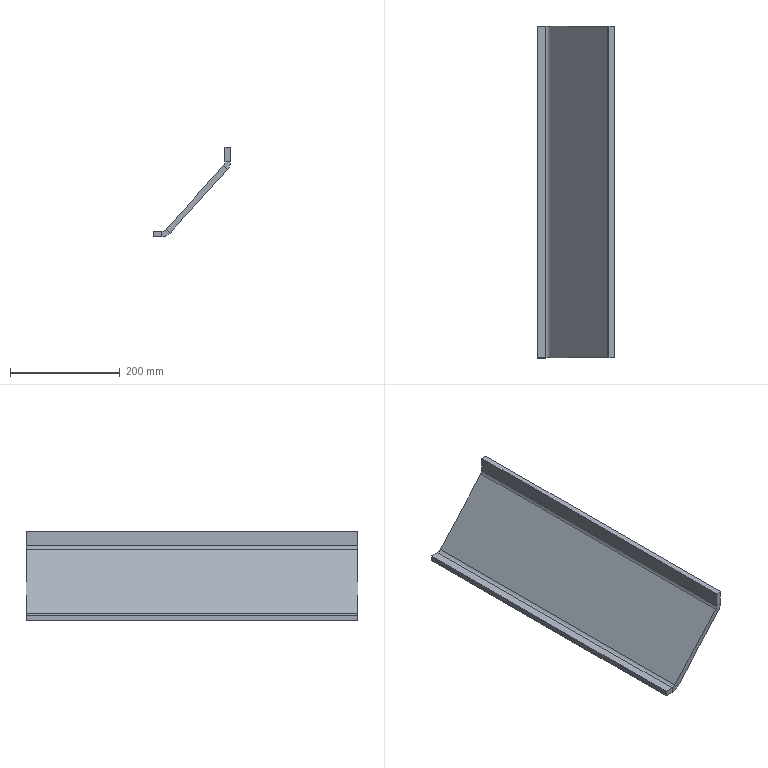Part | SolidWorks | features DelFace 1, DeleteBody 1, FlatPattern 1, FlattenBends 1, MBimport 1, ProcessBends 1, SheetMetal 1 | 1 solid | 22 faces | box 140 x 605 x 163 mm | volume 1343139 mm3 | plane 18 | cylinder 4 | commonest cylinder face diameters 20 x2 40 x2
STEP:
#1=CARTESIAN_POINT('',(500.5,-305.,-1153.));
#2=VERTEX_POINT('',#1);
#3=CARTESIAN_POINT('',(500.5,300.,-1153.));
#4=VERTEX_POINT('',#3);
#5=CARTESIAN_POINT('',(500.5,-305.,-1153.));
#6=DIRECTION('',(0.,1.,0.));
#7=VECTOR('',#6,1000.);
#8=LINE('',#5,#7);
#9=EDGE_CURVE('',#2,#4,#8,.T.);
#10=ORIENTED_EDGE('',*,*,#9,.F.);
#11=CARTESIAN_POINT('',(500.5,-305.,-1143.));
#12=VERTEX_POINT('',#11);
#13=CARTESIAN_POINT('',(500.5,-305.,67.383));
#14=DIRECTION('',(0.,0.,-1.));
#15=VECTOR('',#14,1000.);
#16=LINE('',#13,#15);
#17=EDGE_CURVE('',#12,#2,#16,.T.);
#18=ORIENTED_EDGE('',*,*,#17,.F.);
#19=CARTESIAN_POINT('',(500.5,300.,-1143.));
#20=VERTEX_POINT('',#19);
#21=CARTESIAN_POINT('',(500.5,-305.,-1143.));
#22=DIRECTION('',(0.,1.,0.));
#23=VECTOR('',#22,1000.);
#24=LINE('',#21,#23);
#25=EDGE_CURVE('',#12,#20,#24,.T.);
#26=ORIENTED_EDGE('',*,*,#25,.T.);
#27=CARTESIAN_POINT('',(500.5,300.,67.383));
#28=DIRECTION('',(0.,0.,-1.));
#29=VECTOR('',#28,1000.);
#30=LINE('',#27,#29);
#31=EDGE_CURVE('',#20,#4,#30,.T.);
#32=ORIENTED_EDGE('',*,*,#31,.T.);
#33=EDGE_LOOP('',(#10,#18,#26,#32));
#34=FACE_OUTER_BOUND('',#33,.T.);
#35=CARTESIAN_POINT('',(500.5,-305.,67.383));
#36=DIRECTION('',(-1.,0.,0.));
#37=DIRECTION('',(0.,0.,1.));
#38=AXIS2_PLACEMENT_3D('',#35,#36,#37);
#39=PLANE('',#38);
#40=ADVANCED_FACE('',(#34),#39,.T.);
#41=CARTESIAN_POINT('',(515.725,300.,-1143.));
#42=VERTEX_POINT('',#41);
#43=CARTESIAN_POINT('',(515.725,300.,-1153.));
#44=VERTEX_POINT('',#43);
#45=CARTESIAN_POINT('',(515.725,300.,67.383));
#46=DIRECTION('',(0.,0.,-1.));
#47=VECTOR('',#46,1000.);
#48=LINE('',#45,#47);
#49=EDGE_CURVE('',#42,#44,#48,.T.);
#50=ORIENTED_EDGE('',*,*,#49,.T.);
#51=CARTESIAN_POINT('',(500.5,300.,-1153.));
#52=DIRECTION('',(1.,0.,0.));
#53=VECTOR('',#52,1000.);
#54=LINE('',#51,#53);
#55=EDGE_CURVE('',#4,#44,#54,.T.);
#56=ORIENTED_EDGE('',*,*,#55,.F.);
#57=ORIENTED_EDGE('',*,*,#31,.F.);
#58=CARTESIAN_POINT('',(517.751,300.,-1143.));
#59=DIRECTION('',(-1.,0.,0.));
#60=VECTOR('',#59,1000.);
#61=LINE('',#58,#60);
#62=EDGE_CURVE('',#42,#20,#61,.T.);
#63=ORIENTED_EDGE('',*,*,#62,.F.);
#64=EDGE_LOOP('',(#50,#56,#57,#63));
#65=FACE_OUTER_BOUND('',#64,.T.);
#66=CARTESIAN_POINT('',(517.751,300.,67.383));
#67=DIRECTION('',(0.,-1.,0.));
#68=DIRECTION('',(-0.7431,0.,-0.6691));
#69=AXIS2_PLACEMENT_3D('',#66,#67,#68);
#70=PLANE('',#69);
#71=ADVANCED_FACE('',(#65),#70,.F.);
#72=ORIENTED_EDGE('',*,*,#55,.T.);
#73=CARTESIAN_POINT('',(515.725,-305.,-1153.));
#74=VERTEX_POINT('',#73);
#75=CARTESIAN_POINT('',(515.725,300.,-1153.));
#76=DIRECTION('',(0.,-1.,0.));
#77=VECTOR('',#76,1000.);
#78=LINE('',#75,#77);
#79=EDGE_CURVE('',#44,#74,#78,.T.);
#80=ORIENTED_EDGE('',*,*,#79,.T.);
#81=CARTESIAN_POINT('',(500.5,-305.,-1153.));
#82=DIRECTION('',(1.,0.,0.));
#83=VECTOR('',#82,1000.);
#84=LINE('',#81,#83);
#85=EDGE_CURVE('',#2,#74,#84,.T.);
#86=ORIENTED_EDGE('',*,*,#85,.F.);
#87=ORIENTED_EDGE('',*,*,#9,.T.);
#88=EDGE_LOOP('',(#72,#80,#86,#87));
#89=FACE_OUTER_BOUND('',#88,.T.);
#90=CARTESIAN_POINT('',(500.5,-305.,-1153.));
#91=DIRECTION('',(0.,0.,1.));
#92=DIRECTION('',(1.,0.,0.));
#93=AXIS2_PLACEMENT_3D('',#90,#91,#92);
#94=PLANE('',#93);
#95=ADVANCED_FACE('',(#89),#94,.F.);
#96=ORIENTED_EDGE('',*,*,#85,.T.);
#97=CARTESIAN_POINT('',(515.725,-305.,-1143.));
#98=VERTEX_POINT('',#97);
#99=CARTESIAN_POINT('',(515.725,-305.,67.383));
#100=DIRECTION('',(0.,0.,-1.));
#101=VECTOR('',#100,1000.);
#102=LINE('',#99,#101);
#103=EDGE_CURVE('',#98,#74,#102,.T.);
#104=ORIENTED_EDGE('',*,*,#103,.F.);
#105=CARTESIAN_POINT('',(517.751,-305.,-1143.));
#106=DIRECTION('',(1.,0.,0.));
#107=VECTOR('',#106,1000.);
#108=LINE('',#105,#107);
#109=EDGE_CURVE('',#12,#98,#108,.T.);
#110=ORIENTED_EDGE('',*,*,#109,.F.);
#111=ORIENTED_EDGE('',*,*,#17,.T.);
#112=EDGE_LOOP('',(#96,#104,#110,#111));
#113=FACE_OUTER_BOUND('',#112,.T.);
#114=CARTESIAN_POINT('',(517.751,-305.,67.383));
#115=DIRECTION('',(0.,-1.,0.));
#116=DIRECTION('',(-0.7431,0.,-0.6691));
#117=AXIS2_PLACEMENT_3D('',#114,#115,#116);
#118=PLANE('',#117);
#119=ADVANCED_FACE('',(#113),#118,.T.);
#120=ORIENTED_EDGE('',*,*,#109,.T.);
#121=CARTESIAN_POINT('',(515.725,300.,-1143.));
#122=DIRECTION('',(0.,1.,0.));
#123=VECTOR('',#122,1000.);
#124=LINE('',#121,#123);
#125=EDGE_CURVE('',#98,#42,#124,.T.);
#126=ORIENTED_EDGE('',*,*,#125,.T.);
#127=ORIENTED_EDGE('',*,*,#62,.T.);
#128=ORIENTED_EDGE('',*,*,#25,.F.);
#129=EDGE_LOOP('',(#120,#126,#127,#128));
#130=FACE_OUTER_BOUND('',#129,.T.);
#131=CARTESIAN_POINT('',(517.751,-305.,-1143.));
#132=DIRECTION('',(0.,0.,-1.));
#133=DIRECTION('',(0.,-1.,0.));
#134=AXIS2_PLACEMENT_3D('',#131,#132,#133);
#135=PLANE('',#134);
#136=ADVANCED_FACE('',(#130),#135,.F.);
#137=CARTESIAN_POINT('',(630.5,-305.,-990.));
#138=VERTEX_POINT('',#137);
#139=CARTESIAN_POINT('',(640.5,-305.,-990.));
#140=VERTEX_POINT('',#139);
#141=CARTESIAN_POINT('',(-580.672,-305.,-990.));
#142=DIRECTION('',(1.,0.,0.));
#143=VECTOR('',#142,1000.);
#144=LINE('',#141,#143);
#145=EDGE_CURVE('',#138,#140,#144,.T.);
#146=ORIENTED_EDGE('',*,*,#145,.T.);
#147=CARTESIAN_POINT('',(640.5,300.,-990.));
#148=VERTEX_POINT('',#147);
#149=CARTESIAN_POINT('',(640.5,-305.,-990.));
#150=DIRECTION('',(0.,1.,0.));
#151=VECTOR('',#150,1000.);
#152=LINE('',#149,#151);
#153=EDGE_CURVE('',#140,#148,#152,.T.);
#154=ORIENTED_EDGE('',*,*,#153,.T.);
#155=CARTESIAN_POINT('',(630.5,300.,-990.));
#156=VERTEX_POINT('',#155);
#157=CARTESIAN_POINT('',(-580.672,300.,-990.));
#158=DIRECTION('',(1.,0.,0.));
#159=VECTOR('',#158,1000.);
#160=LINE('',#157,#159);
#161=EDGE_CURVE('',#156,#148,#160,.T.);
#162=ORIENTED_EDGE('',*,*,#161,.F.);
#163=CARTESIAN_POINT('',(630.5,-305.,-990.));
#164=DIRECTION('',(0.,1.,0.));
#165=VECTOR('',#164,1000.);
#166=LINE('',#163,#165);
#167=EDGE_CURVE('',#138,#156,#166,.T.);
#168=ORIENTED_EDGE('',*,*,#167,.F.);
#169=EDGE_LOOP('',(#146,#154,#162,#168));
#170=FACE_OUTER_BOUND('',#169,.T.);
#171=CARTESIAN_POINT('',(-580.672,-305.,-990.));
#172=DIRECTION('',(0.,0.,-1.));
#173=DIRECTION('',(-1.,0.,0.));
#174=AXIS2_PLACEMENT_3D('',#171,#172,#173);
#175=PLANE('',#174);
#176=ADVANCED_FACE('',(#170),#175,.F.);
#177=CARTESIAN_POINT('',(640.5,-305.,-1016.636));
#178=VERTEX_POINT('',#177);
#179=CARTESIAN_POINT('',(640.5,-305.,-1016.314));
#180=DIRECTION('',(0.,0.,1.));
#181=VECTOR('',#180,1000.);
#182=LINE('',#179,#181);
#183=EDGE_CURVE('',#178,#140,#182,.T.);
#184=ORIENTED_EDGE('',*,*,#183,.T.);
#185=ORIENTED_EDGE('',*,*,#145,.F.);
#186=CARTESIAN_POINT('',(630.5,-305.,-1016.636));
#187=VERTEX_POINT('',#186);
#188=CARTESIAN_POINT('',(630.5,-305.,-990.));
#189=DIRECTION('',(0.,0.,-1.));
#190=VECTOR('',#189,1000.);
#191=LINE('',#188,#190);
#192=EDGE_CURVE('',#138,#187,#191,.T.);
#193=ORIENTED_EDGE('',*,*,#192,.T.);
#194=CARTESIAN_POINT('',(-580.672,-305.,-1016.636));
#195=DIRECTION('',(1.,0.,0.));
#196=VECTOR('',#195,1000.);
#197=LINE('',#194,#196);
#198=EDGE_CURVE('',#187,#178,#197,.T.);
#199=ORIENTED_EDGE('',*,*,#198,.T.);
#200=EDGE_LOOP('',(#184,#185,#193,#199));
#201=FACE_OUTER_BOUND('',#200,.T.);
#202=CARTESIAN_POINT('',(-580.672,-305.,-990.));
#203=DIRECTION('',(0.,-1.,0.));
#204=DIRECTION('',(0.6691,0.,-0.7431));
#205=AXIS2_PLACEMENT_3D('',#202,#203,#204);
#206=PLANE('',#205);
#207=ADVANCED_FACE('',(#201),#206,.T.);
#208=ORIENTED_EDGE('',*,*,#183,.F.);
#209=CARTESIAN_POINT('',(640.5,300.,-1016.636));
#210=VERTEX_POINT('',#209);
#211=CARTESIAN_POINT('',(640.5,-305.,-1016.636));
#212=DIRECTION('',(0.,1.,0.));
#213=VECTOR('',#212,1000.);
#214=LINE('',#211,#213);
#215=EDGE_CURVE('',#178,#210,#214,.T.);
#216=ORIENTED_EDGE('',*,*,#215,.T.);
#217=CARTESIAN_POINT('',(640.5,300.,-990.));
#218=DIRECTION('',(0.,0.,-1.));
#219=VECTOR('',#218,1000.);
#220=LINE('',#217,#219);
#221=EDGE_CURVE('',#148,#210,#220,.T.);
#222=ORIENTED_EDGE('',*,*,#221,.F.);
#223=ORIENTED_EDGE('',*,*,#153,.F.);
#224=EDGE_LOOP('',(#208,#216,#222,#223));
#225=FACE_OUTER_BOUND('',#224,.T.);
#226=CARTESIAN_POINT('',(640.5,-305.,-1016.314));
#227=DIRECTION('',(-1.,0.,0.));
#228=DIRECTION('',(0.,0.,1.));
#229=AXIS2_PLACEMENT_3D('',#226,#227,#228);
#230=PLANE('',#229);
#231=ADVANCED_FACE('',(#225),#230,.F.);
#232=ORIENTED_EDGE('',*,*,#161,.T.);
#233=ORIENTED_EDGE('',*,*,#221,.T.);
#234=CARTESIAN_POINT('',(630.5,300.,-1016.636));
#235=VERTEX_POINT('',#234);
#236=CARTESIAN_POINT('',(-580.672,300.,-1016.636));
#237=DIRECTION('',(1.,0.,0.));
#238=VECTOR('',#237,1000.);
#239=LINE('',#236,#238);
#240=EDGE_CURVE('',#235,#210,#239,.T.);
#241=ORIENTED_EDGE('',*,*,#240,.F.);
#242=CARTESIAN_POINT('',(630.5,300.,-990.));
#243=DIRECTION('',(0.,0.,-1.));
#244=VECTOR('',#243,1000.);
#245=LINE('',#242,#244);
#246=EDGE_CURVE('',#156,#235,#245,.T.);
#247=ORIENTED_EDGE('',*,*,#246,.F.);
#248=EDGE_LOOP('',(#232,#233,#241,#247));
#249=FACE_OUTER_BOUND('',#248,.T.);
#250=CARTESIAN_POINT('',(-580.672,300.,-990.));
#251=DIRECTION('',(0.,-1.,0.));
#252=DIRECTION('',(0.6691,0.,-0.7431));
#253=AXIS2_PLACEMENT_3D('',#250,#251,#252);
#254=PLANE('',#253);
#255=ADVANCED_FACE('',(#249),#254,.F.);
#256=ORIENTED_EDGE('',*,*,#246,.T.);
#257=CARTESIAN_POINT('',(630.5,-305.,-1016.636));
#258=DIRECTION('',(0.,-1.,0.));
#259=VECTOR('',#258,1000.);
#260=LINE('',#257,#259);
#261=EDGE_CURVE('',#235,#187,#260,.T.);
#262=ORIENTED_EDGE('',*,*,#261,.T.);
#263=ORIENTED_EDGE('',*,*,#192,.F.);
#264=ORIENTED_EDGE('',*,*,#167,.T.);
#265=EDGE_LOOP('',(#256,#262,#263,#264));
#266=FACE_OUTER_BOUND('',#265,.T.);
#267=CARTESIAN_POINT('',(630.5,-305.,-990.));
#268=DIRECTION('',(1.,0.,0.));
#269=DIRECTION('',(0.,1.,0.));
#270=AXIS2_PLACEMENT_3D('',#267,#268,#269);
#271=PLANE('',#270);
#272=ADVANCED_FACE('',(#266),#271,.F.);
#273=CARTESIAN_POINT('',(627.931,300.,-1023.327));
#274=VERTEX_POINT('',#273);
#275=CARTESIAN_POINT('',(635.363,300.,-1030.019));
#276=VERTEX_POINT('',#275);
#277=CARTESIAN_POINT('',(-300.902,300.,-187.001));
#278=DIRECTION('',(0.7431,0.,-0.6691));
#279=VECTOR('',#278,1000.);
#280=LINE('',#277,#279);
#281=EDGE_CURVE('',#274,#276,#280,.T.);
#282=ORIENTED_EDGE('',*,*,#281,.T.);
#283=CARTESIAN_POINT('',(530.588,300.,-1146.383));
#284=VERTEX_POINT('',#283);
#285=CARTESIAN_POINT('',(529.984,300.,-1147.053));
#286=DIRECTION('',(0.6691,0.,0.7431));
#287=VECTOR('',#286,1000.);
#288=LINE('',#285,#287);
#289=EDGE_CURVE('',#284,#276,#288,.T.);
#290=ORIENTED_EDGE('',*,*,#289,.F.);
#291=CARTESIAN_POINT('',(523.157,300.,-1139.691));
#292=VERTEX_POINT('',#291);
#293=CARTESIAN_POINT('',(-405.677,300.,-303.365));
#294=DIRECTION('',(0.7431,0.,-0.6691));
#295=VECTOR('',#294,1000.);
#296=LINE('',#293,#295);
#297=EDGE_CURVE('',#292,#284,#296,.T.);
#298=ORIENTED_EDGE('',*,*,#297,.F.);
#299=CARTESIAN_POINT('',(630.33,300.,-1020.663));
#300=DIRECTION('',(-0.6691,0.,-0.7431));
#301=VECTOR('',#300,1000.);
#302=LINE('',#299,#301);
#303=EDGE_CURVE('',#274,#292,#302,.T.);
#304=ORIENTED_EDGE('',*,*,#303,.F.);
#305=EDGE_LOOP('',(#282,#290,#298,#304));
#306=FACE_OUTER_BOUND('',#305,.T.);
#307=CARTESIAN_POINT('',(-298.503,300.,-184.337));
#308=DIRECTION('',(0.,-1.,0.));
#309=DIRECTION('',(0.,0.,-1.));
#310=AXIS2_PLACEMENT_3D('',#307,#308,#309);
#311=PLANE('',#310);
#312=ADVANCED_FACE('',(#306),#311,.F.);
#313=CARTESIAN_POINT('',(530.588,-305.,-1146.383));
#314=VERTEX_POINT('',#313);
#315=CARTESIAN_POINT('',(635.363,-305.,-1030.019));
#316=VERTEX_POINT('',#315);
#317=CARTESIAN_POINT('',(529.984,-305.,-1147.053));
#318=DIRECTION('',(0.6691,0.,0.7431));
#319=VECTOR('',#318,1000.);
#320=LINE('',#317,#319);
#321=EDGE_CURVE('',#314,#316,#320,.T.);
#322=ORIENTED_EDGE('',*,*,#321,.T.);
#323=CARTESIAN_POINT('',(627.931,-305.,-1023.327));
#324=VERTEX_POINT('',#323);
#325=CARTESIAN_POINT('',(-300.902,-305.,-187.001));
#326=DIRECTION('',(0.7431,0.,-0.6691));
#327=VECTOR('',#326,1000.);
#328=LINE('',#325,#327);
#329=EDGE_CURVE('',#324,#316,#328,.T.);
#330=ORIENTED_EDGE('',*,*,#329,.F.);
#331=CARTESIAN_POINT('',(523.157,-305.,-1139.691));
#332=VERTEX_POINT('',#331);
#333=CARTESIAN_POINT('',(630.33,-305.,-1020.663));
#334=DIRECTION('',(-0.6691,0.,-0.7431));
#335=VECTOR('',#334,1000.);
#336=LINE('',#333,#335);
#337=EDGE_CURVE('',#324,#332,#336,.T.);
#338=ORIENTED_EDGE('',*,*,#337,.T.);
#339=CARTESIAN_POINT('',(-405.677,-305.,-303.365));
#340=DIRECTION('',(0.7431,0.,-0.6691));
#341=VECTOR('',#340,1000.);
#342=LINE('',#339,#341);
#343=EDGE_CURVE('',#332,#314,#342,.T.);
#344=ORIENTED_EDGE('',*,*,#343,.T.);
#345=EDGE_LOOP('',(#322,#330,#338,#344));
#346=FACE_OUTER_BOUND('',#345,.T.);
#347=CARTESIAN_POINT('',(-298.503,-305.,-184.337));
#348=DIRECTION('',(0.,-1.,0.));
#349=DIRECTION('',(0.,0.,-1.));
#350=AXIS2_PLACEMENT_3D('',#347,#348,#349);
#351=PLANE('',#350);
#352=ADVANCED_FACE('',(#346),#351,.T.);
#353=CARTESIAN_POINT('',(523.157,300.,-1139.691));
#354=DIRECTION('',(0.,1.,0.));
#355=VECTOR('',#354,1000.);
#356=LINE('',#353,#355);
#357=EDGE_CURVE('',#332,#292,#356,.T.);
#358=ORIENTED_EDGE('',*,*,#357,.F.);
#359=ORIENTED_EDGE('',*,*,#337,.F.);
#360=CARTESIAN_POINT('',(627.931,-305.,-1023.327));
#361=DIRECTION('',(0.,-1.,0.));
#362=VECTOR('',#361,1000.);
#363=LINE('',#360,#362);
#364=EDGE_CURVE('',#274,#324,#363,.T.);
#365=ORIENTED_EDGE('',*,*,#364,.F.);
#366=ORIENTED_EDGE('',*,*,#303,.T.);
#367=EDGE_LOOP('',(#358,#359,#365,#366));
#368=FACE_OUTER_BOUND('',#367,.T.);
#369=CARTESIAN_POINT('',(630.33,-305.,-1020.663));
#370=DIRECTION('',(0.7431,0.,-0.6691));
#371=DIRECTION('',(0.,-1.,0.));
#372=AXIS2_PLACEMENT_3D('',#369,#370,#371);
#373=PLANE('',#372);
#374=ADVANCED_FACE('',(#368),#373,.F.);
#375=CARTESIAN_POINT('',(530.588,300.,-1146.383));
#376=DIRECTION('',(0.,-1.,0.));
#377=VECTOR('',#376,1000.);
#378=LINE('',#375,#377);
#379=EDGE_CURVE('',#284,#314,#378,.T.);
#380=ORIENTED_EDGE('',*,*,#379,.F.);
#381=ORIENTED_EDGE('',*,*,#289,.T.);
#382=CARTESIAN_POINT('',(635.363,-305.,-1030.019));
#383=DIRECTION('',(0.,1.,0.));
#384=VECTOR('',#383,1000.);
#385=LINE('',#382,#384);
#386=EDGE_CURVE('',#316,#276,#385,.T.);
#387=ORIENTED_EDGE('',*,*,#386,.F.);
#388=ORIENTED_EDGE('',*,*,#321,.F.);
#389=EDGE_LOOP('',(#380,#381,#387,#388));
#390=FACE_OUTER_BOUND('',#389,.T.);
#391=CARTESIAN_POINT('',(529.984,-305.,-1147.053));
#392=DIRECTION('',(-0.7431,0.,0.6691));
#393=DIRECTION('',(0.,1.,0.));
#394=AXIS2_PLACEMENT_3D('',#391,#392,#393);
#395=PLANE('',#394);
#396=ADVANCED_FACE('',(#390),#395,.F.);
#397=ORIENTED_EDGE('',*,*,#198,.F.);
#398=CARTESIAN_POINT('',(620.5,-305.,-1016.636));
#399=DIRECTION('',(0.,1.,0.));
#400=DIRECTION('',(0.,0.,1.));
#401=AXIS2_PLACEMENT_3D('',#398,#399,#400);
#402=CIRCLE('',#401,10.);
#403=EDGE_CURVE('',#187,#324,#402,.T.);
#404=ORIENTED_EDGE('',*,*,#403,.T.);
#405=ORIENTED_EDGE('',*,*,#329,.T.);
#406=CARTESIAN_POINT('',(620.5,-305.,-1016.636));
#407=DIRECTION('',(0.,1.,0.));
#408=DIRECTION('',(0.,0.,1.));
#409=AXIS2_PLACEMENT_3D('',#406,#407,#408);
#410=CIRCLE('',#409,20.);
#411=EDGE_CURVE('',#178,#316,#410,.T.);
#412=ORIENTED_EDGE('',*,*,#411,.F.);
#413=EDGE_LOOP('',(#397,#404,#405,#412));
#414=FACE_OUTER_BOUND('',#413,.T.);
#415=CARTESIAN_POINT('',(620.5,-305.,-1016.636));
#416=DIRECTION('',(0.,-1.,0.));
#417=DIRECTION('',(1.,0.,0.));
#418=AXIS2_PLACEMENT_3D('',#415,#416,#417);
#419=PLANE('',#418);
#420=ADVANCED_FACE('',(#414),#419,.T.);
#421=CARTESIAN_POINT('',(620.5,300.,-1016.636));
#422=DIRECTION('',(0.,-1.,0.));
#423=DIRECTION('',(0.,0.,1.));
#424=AXIS2_PLACEMENT_3D('',#421,#422,#423);
#425=CIRCLE('',#424,10.);
#426=EDGE_CURVE('',#274,#235,#425,.T.);
#427=ORIENTED_EDGE('',*,*,#426,.T.);
#428=ORIENTED_EDGE('',*,*,#240,.T.);
#429=CARTESIAN_POINT('',(620.5,300.,-1016.636));
#430=DIRECTION('',(0.,-1.,0.));
#431=DIRECTION('',(0.,0.,1.));
#432=AXIS2_PLACEMENT_3D('',#429,#430,#431);
#433=CIRCLE('',#432,20.);
#434=EDGE_CURVE('',#276,#210,#433,.T.);
#435=ORIENTED_EDGE('',*,*,#434,.F.);
#436=ORIENTED_EDGE('',*,*,#281,.F.);
#437=EDGE_LOOP('',(#427,#428,#435,#436));
#438=FACE_OUTER_BOUND('',#437,.T.);
#439=CARTESIAN_POINT('',(620.5,300.,-1016.636));
#440=DIRECTION('',(0.,1.,0.));
#441=DIRECTION('',(-1.,0.,0.));
#442=AXIS2_PLACEMENT_3D('',#439,#440,#441);
#443=PLANE('',#442);
#444=ADVANCED_FACE('',(#438),#443,.T.);
#445=ORIENTED_EDGE('',*,*,#386,.T.);
#446=ORIENTED_EDGE('',*,*,#434,.T.);
#447=ORIENTED_EDGE('',*,*,#215,.F.);
#448=ORIENTED_EDGE('',*,*,#411,.T.);
#449=EDGE_LOOP('',(#445,#446,#447,#448));
#450=FACE_OUTER_BOUND('',#449,.T.);
#451=CARTESIAN_POINT('',(620.5,-952.941,-1016.636));
#452=DIRECTION('',(0.,1.,0.));
#453=DIRECTION('',(0.,0.,1.));
#454=AXIS2_PLACEMENT_3D('',#451,#452,#453);
#455=CYLINDRICAL_SURFACE('',#454,20.);
#456=ADVANCED_FACE('',(#450),#455,.T.);
#457=ORIENTED_EDGE('',*,*,#364,.T.);
#458=ORIENTED_EDGE('',*,*,#403,.F.);
#459=ORIENTED_EDGE('',*,*,#261,.F.);
#460=ORIENTED_EDGE('',*,*,#426,.F.);
#461=EDGE_LOOP('',(#457,#458,#459,#460));
#462=FACE_OUTER_BOUND('',#461,.T.);
#463=CARTESIAN_POINT('',(620.5,-952.941,-1016.636));
#464=DIRECTION('',(0.,1.,0.));
#465=DIRECTION('',(0.,0.,1.));
#466=AXIS2_PLACEMENT_3D('',#463,#464,#465);
#467=CYLINDRICAL_SURFACE('',#466,10.);
#468=ADVANCED_FACE('',(#462),#467,.F.);
#469=ORIENTED_EDGE('',*,*,#49,.F.);
#470=CARTESIAN_POINT('',(515.725,300.,-1133.));
#471=DIRECTION('',(0.,-1.,0.));
#472=DIRECTION('',(0.,0.,-1.));
#473=AXIS2_PLACEMENT_3D('',#470,#471,#472);
#474=CIRCLE('',#473,10.);
#475=EDGE_CURVE('',#42,#292,#474,.T.);
#476=ORIENTED_EDGE('',*,*,#475,.T.);
#477=ORIENTED_EDGE('',*,*,#297,.T.);
#478=CARTESIAN_POINT('',(515.725,300.,-1133.));
#479=DIRECTION('',(0.,-1.,0.));
#480=DIRECTION('',(0.,0.,-1.));
#481=AXIS2_PLACEMENT_3D('',#478,#479,#480);
#482=CIRCLE('',#481,20.);
#483=EDGE_CURVE('',#44,#284,#482,.T.);
#484=ORIENTED_EDGE('',*,*,#483,.F.);
#485=EDGE_LOOP('',(#469,#476,#477,#484));
#486=FACE_OUTER_BOUND('',#485,.T.);
#487=CARTESIAN_POINT('',(515.725,300.,-1133.));
#488=DIRECTION('',(0.,1.,0.));
#489=DIRECTION('',(0.,0.,1.));
#490=AXIS2_PLACEMENT_3D('',#487,#488,#489);
#491=PLANE('',#490);
#492=ADVANCED_FACE('',(#486),#491,.T.);
#493=CARTESIAN_POINT('',(515.725,-305.,-1133.));
#494=DIRECTION('',(0.,1.,0.));
#495=DIRECTION('',(0.,0.,-1.));
#496=AXIS2_PLACEMENT_3D('',#493,#494,#495);
#497=CIRCLE('',#496,10.);
#498=EDGE_CURVE('',#332,#98,#497,.T.);
#499=ORIENTED_EDGE('',*,*,#498,.T.);
#500=ORIENTED_EDGE('',*,*,#103,.T.);
#501=CARTESIAN_POINT('',(515.725,-305.,-1133.));
#502=DIRECTION('',(0.,1.,0.));
#503=DIRECTION('',(0.,0.,-1.));
#504=AXIS2_PLACEMENT_3D('',#501,#502,#503);
#505=CIRCLE('',#504,20.);
#506=EDGE_CURVE('',#314,#74,#505,.T.);
#507=ORIENTED_EDGE('',*,*,#506,.F.);
#508=ORIENTED_EDGE('',*,*,#343,.F.);
#509=EDGE_LOOP('',(#499,#500,#507,#508));
#510=FACE_OUTER_BOUND('',#509,.T.);
#511=CARTESIAN_POINT('',(515.725,-305.,-1133.));
#512=DIRECTION('',(0.,-1.,0.));
#513=DIRECTION('',(0.,0.,-1.));
#514=AXIS2_PLACEMENT_3D('',#511,#512,#513);
#515=PLANE('',#514);
#516=ADVANCED_FACE('',(#510),#515,.T.);
#517=ORIENTED_EDGE('',*,*,#379,.T.);
#518=ORIENTED_EDGE('',*,*,#506,.T.);
#519=ORIENTED_EDGE('',*,*,#79,.F.);
#520=ORIENTED_EDGE('',*,*,#483,.T.);
#521=EDGE_LOOP('',(#517,#518,#519,#520));
#522=FACE_OUTER_BOUND('',#521,.T.);
#523=CARTESIAN_POINT('',(515.725,944.861,-1133.));
#524=DIRECTION('',(0.,-1.,0.));
#525=DIRECTION('',(0.,0.,-1.));
#526=AXIS2_PLACEMENT_3D('',#523,#524,#525);
#527=CYLINDRICAL_SURFACE('',#526,20.);
#528=ADVANCED_FACE('',(#522),#527,.T.);
#529=ORIENTED_EDGE('',*,*,#357,.T.);
#530=ORIENTED_EDGE('',*,*,#475,.F.);
#531=ORIENTED_EDGE('',*,*,#125,.F.);
#532=ORIENTED_EDGE('',*,*,#498,.F.);
#533=EDGE_LOOP('',(#529,#530,#531,#532));
#534=FACE_OUTER_BOUND('',#533,.T.);
#535=CARTESIAN_POINT('',(515.725,944.861,-1133.));
#536=DIRECTION('',(0.,-1.,0.));
#537=DIRECTION('',(0.,0.,-1.));
#538=AXIS2_PLACEMENT_3D('',#535,#536,#537);
#539=CYLINDRICAL_SURFACE('',#538,10.);
#540=ADVANCED_FACE('',(#534),#539,.F.);
#541=CLOSED_SHELL('',(#40,#71,#95,#119,#136,#176,#207,#231,#255,#272,#312,#352,#374,#396,#420,#444,#456,#468,#492,#516,#528,#540));
#542=MANIFOLD_SOLID_BREP('',#541);
#543=CARTESIAN_POINT('',(0.,0.,0.));
#544=DIRECTION('',(0.,0.,1.));
#545=DIRECTION('',(1.,0.,0.));
#546=AXIS2_PLACEMENT_3D('',#543,#544,#545);
#547=(LENGTH_UNIT()NAMED_UNIT(*)SI_UNIT(.MILLI.,.METRE.));
#548=UNCERTAINTY_MEASURE_WITH_UNIT(LENGTH_MEASURE(0.00001),#547,'','');
#549=(NAMED_UNIT(*)PLANE_ANGLE_UNIT()SI_UNIT($,.RADIAN.));
#550=(NAMED_UNIT(*)SI_UNIT($,.STERADIAN.)SOLID_ANGLE_UNIT());
#551=(GEOMETRIC_REPRESENTATION_CONTEXT(3)GLOBAL_UNCERTAINTY_ASSIGNED_CONTEXT((#548))GLOBAL_UNIT_ASSIGNED_CONTEXT((#547,#549,#550))REPRESENTATION_CONTEXT('',''));
#552=ADVANCED_BREP_SHAPE_REPRESENTATION('',(#542,#546),#551);